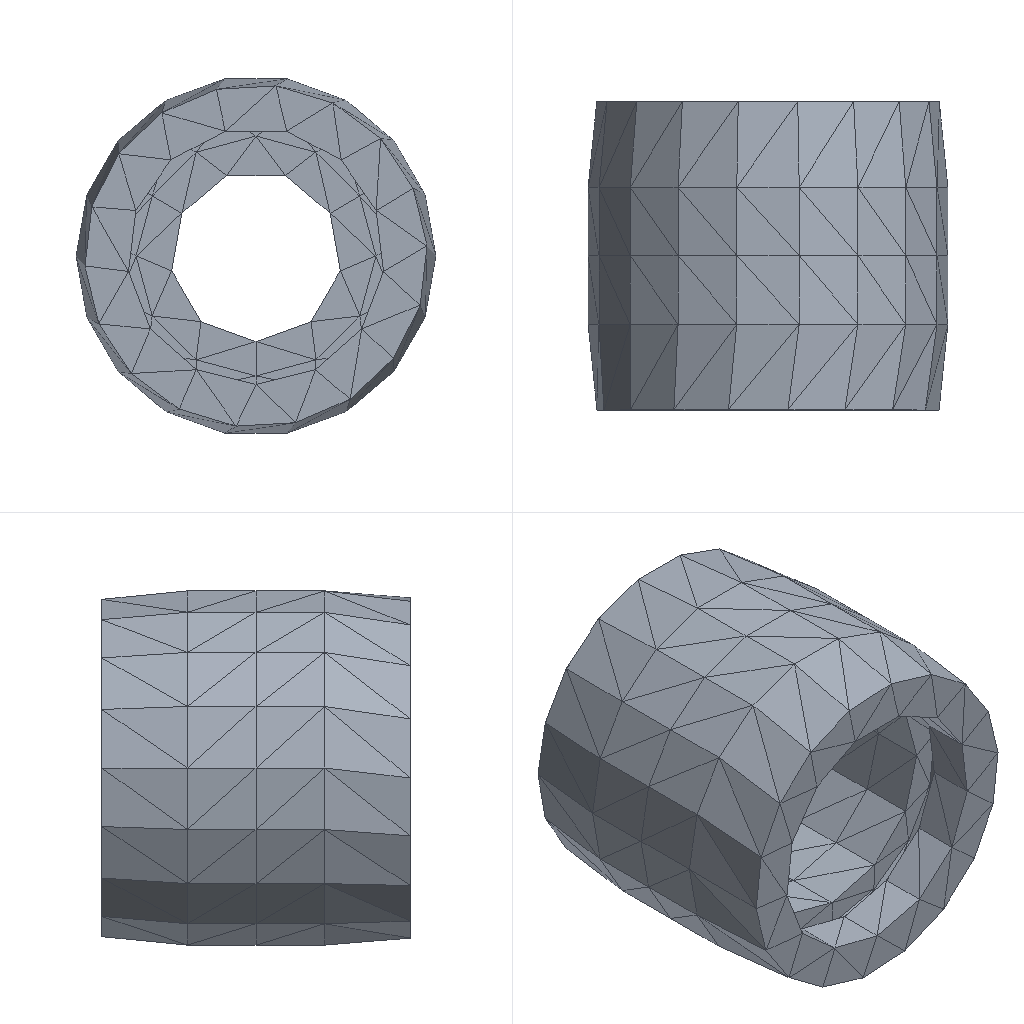Simulation study | nx simcenter
Set-up summary:
category,name,step,type,value,unit,region
solver,nx_nastran (Simcenter)
units,not stated in the deck,,not stated
analysis,deck,,static,static
analysis,solution,,SOL,101
load_step,SUBCASE 1,1,SUBCASE,SPC=1 LOAD=2
load_step,requested,,,1
mesh,nodes,,,1271
mesh,elements,,,606
element_type,CTETRA,,solid,606
load,nodal force total,,FX,0.0,model units
load,nodal force total,,FY,0.0,model units
load,nodal force total,,FZ,-1999999.99,model units
load,load commands in deck,,count,144
bc,support commands in deck,,count,180
analysis,NX solution 0,,Structural,Linear Statics - Single Constraint
check,setup vs results,,match,every grid point's frame and coordinates and every element id; grid points of CTETRA elements
Nastran input file, long lists of numbers shortened:
$*$$$$$$$$$$$$$$$$$$$$$$$$$$$$$$$$$$$$$$$$$$$$$$$$$$$$$$$$$$$$$$$$$
$*
$*                    NX v10.0.0.24 TRANSLATOR
$*                    FOR NX NASTRAN VERSION 10.0
$ (33 more lines like these left out)
ASSIGN OUTPUT2='147_sim1-solution_1.op2' UNIT=12
$*
$*$$$$$$$$$$$$$$$$$$$$$$$$$$$$$$$$$$$
$*
$* EXECUTIVE CONTROL
$*
$*$$$$$$$$$$$$$$$$$$$$$$$$$$$$$$$$$$$
$*
ID,NASTRAN,147_sim1-solution_1
SOL 101
CEND
$*
$*$$$$$$$$$$$$$$$$$$$$$$$$$$$$$$$$$$$
$*
$* CASE CONTROL
$*
$*$$$$$$$$$$$$$$$$$$$$$$$$$$$$$$$$$$$
$*
TITLE = Solution 1
ECHO = NONE
SPC = 1
OUTPUT
BCRESULTS(TRACTION,FORCE,PLOT) = ALL
DISPLACEMENT(PLOT) = ALL
ESE(PLOT) = ALL
FORCE(PLOT,CORNER) = ALL
OLOAD(PLOT) = ALL
SPCFORCES(PLOT) = ALL
STRAIN(PLOT,FIBER,CORNER) = ALL
STRESS(PLOT,CORNER) = ALL
$*  NX Step: Subcase - Static Loads 1
SUBCASE 1
LABEL = Subcase - Static Loads 1
LOAD = 2
$*
$*$$$$$$$$$$$$$$$$$$$$$$$$$$$$$$$$$$$
$*
$* BULK DATA
$*
$*$$$$$$$$$$$$$$$$$$$$$$$$$$$$$$$$$$$
$*
BEGIN BULK
$*
$* PARAM CARDS
$*
PARAM      K6ROT100.0000
PARAM     OIBULK     YES
PARAM    OMACHPR     YES
PARAM       POST      -2
PARAM    POSTEXT     YES
PARAM    UNITSYS   MN-MM
$*
$* GRID CARDS
$*
GRID*               1259               00.0000000000E+00-1.754299927E+01+
*       -7.500000000E+00               0
GRID*               1260               00.0000000000E+00-1.482100010E+01+
*       -7.500000000E+00               0
$ (2538 more lines like these left out)
$*
$* ELEMENT CARDS
$*
$*  NX Mesh Collector: Solid(1)
$*  NX Mesh: 3d_mesh(1)
CTETRA         1       1     644    1132     535    1133     746       2+
+              3     747    1151       4
CTETRA         2       1    1098     546       1    1097       5       6+
+              7    1100       8       9
$ (1208 more lines like these left out)
$*
$* PROPERTY CARDS
$*
$*  NX Property: PSOLID1
PSOLID         1       2       0                           SMECH
$*
$* MATERIAL CARDS
$*
$*  NX Material: 45
MAT1           22.1000+8        0.3100007.8500-61.7280-5
$*
$* LOAD AND CONSTRAINT CARDS
$*
$*  NX Load and Constraint: Fixed(1)
SPC            1     643  123456  0.0000
SPC            1     644  123456  0.0000
SPC            1     645  123456  0.0000
SPC            1     646  123456  0.0000
$ (176 more lines like these left out)
$*  NX Load and Constraint: Force(1)
FORCE          2     830       018385.67  0.0000  0.0000-1.00000
FORCE          2     831       018516.13  0.0000  0.0000-1.00000
FORCE          2     832       018657.52  0.0000  0.0000-1.00000
FORCE          2     833       018523.76  0.0000  0.0000-1.00000
$ (140 more lines like these left out)
ENDDATA f395ac20
Results summary:
result,analysis,,,static
result,last_loadstep,,,1
result,primary field,,,displacements
result,reaction total,,FX,-0.004883,model units
result,reaction total,,FY,-0.003395,model units
result,reaction total,,FZ,2000000.0,model units
result,NX solution 0,,loadcases,1,mm